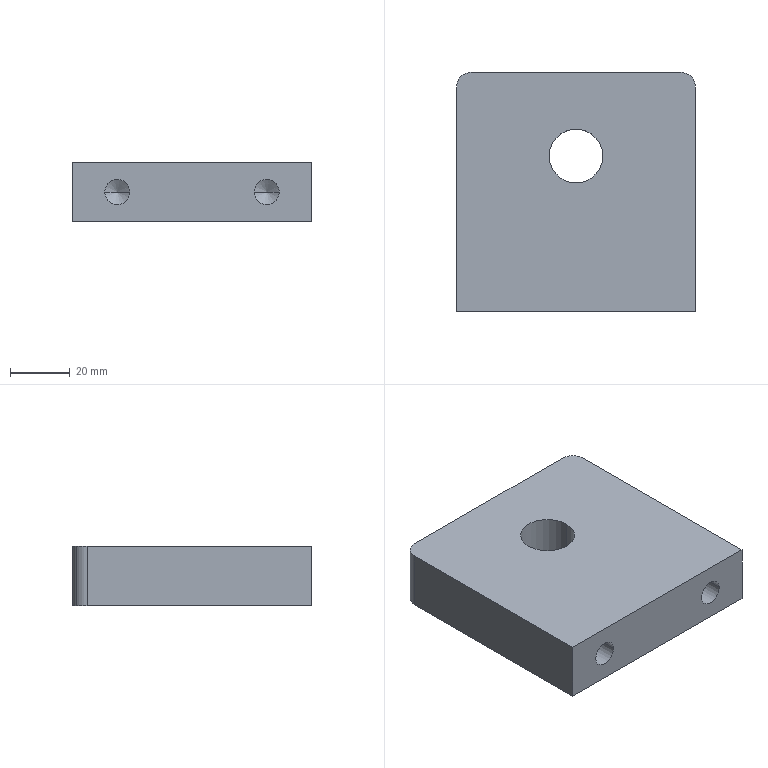Part | STEP file | DCV-000-032 | 1 solid | 20 faces | box 80 x 80 x 20 mm | volume 119595 mm3 | cylinder 10 | plane 6 | cone 4 | commonest cylinder face diameters 8.376 x4 10 x4 18 x2
STEP:
#1=CARTESIAN_POINT('',(0.,0.,0.));
#2=DIRECTION('',(0.,0.,1.));
#3=DIRECTION('',(1.,0.,0.));
#4=AXIS2_PLACEMENT_3D('',#1,#2,#3);
#5=CARTESIAN_POINT('',(40.,75.,0.));
#6=VERTEX_POINT('',#5);
#7=CARTESIAN_POINT('',(38.536,78.536,0.));
#8=VERTEX_POINT('',#7);
#9=CARTESIAN_POINT('',(35.,75.,0.));
#10=DIRECTION('',(0.,0.,1.));
#11=DIRECTION('',(0.7071,0.7071,0.));
#12=AXIS2_PLACEMENT_3D('',#9,#10,#11);
#13=CIRCLE('',#12,5.);
#14=CARTESIAN_POINT('',(35.,75.,0.));
#15=DIRECTION('',(0.,0.,1.));
#16=DIRECTION('',(0.7071,0.7071,0.));
#17=AXIS2_PLACEMENT_3D('',#14,#15,#16);
#18=CYLINDRICAL_SURFACE('',#17,5.);
#19=CARTESIAN_POINT('',(0.,0.));
#20=DIRECTION('',(1.,0.));
#21=VECTOR('',#20,1.);
#22=LINE('',#19,#21);
#23=(GEOMETRIC_REPRESENTATION_CONTEXT(2)PARAMETRIC_REPRESENTATION_CONTEXT()REPRESENTATION_CONTEXT('',''));
#24=DEFINITIONAL_REPRESENTATION('',(#22),#23);
#25=PCURVE('',#18,#24);
#26=CARTESIAN_POINT('',(0.,40.,0.));
#27=DIRECTION('',(0.,0.,1.));
#28=DIRECTION('',(1.,0.,0.));
#29=AXIS2_PLACEMENT_3D('',#26,#27,#28);
#30=PLANE('',#29);
#31=CARTESIAN_POINT('',(35.,35.));
#32=DIRECTION('',(0.7071,0.7071));
#33=AXIS2_PLACEMENT_2D('',#31,#32);
#34=CIRCLE('',#33,5.);
#35=(GEOMETRIC_REPRESENTATION_CONTEXT(2)PARAMETRIC_REPRESENTATION_CONTEXT()REPRESENTATION_CONTEXT('',''));
#36=DEFINITIONAL_REPRESENTATION('',(#34),#35);
#37=PCURVE('',#30,#36);
#38=SURFACE_CURVE('',#13,(#25,#37),.PCURVE_S1.);
#39=EDGE_CURVE('',#6,#8,#38,.T.);
#40=ORIENTED_EDGE('',*,*,#39,.T.);
#41=CARTESIAN_POINT('',(38.536,78.536,20.));
#42=VERTEX_POINT('',#41);
#43=CARTESIAN_POINT('',(38.536,78.536,0.));
#44=DIRECTION('',(0.,0.,1.));
#45=VECTOR('',#44,1.);
#46=LINE('',#43,#45);
#47=CARTESIAN_POINT('',(6.283,0.));
#48=DIRECTION('',(0.,1.));
#49=VECTOR('',#48,1.);
#50=LINE('',#47,#49);
#51=(GEOMETRIC_REPRESENTATION_CONTEXT(2)PARAMETRIC_REPRESENTATION_CONTEXT()REPRESENTATION_CONTEXT('',''));
#52=DEFINITIONAL_REPRESENTATION('',(#50),#51);
#53=PCURVE('',#18,#52);
#54=CARTESIAN_POINT('',(35.,75.,0.));
#55=DIRECTION('',(0.,0.,1.));
#56=DIRECTION('',(0.7071,0.7071,0.));
#57=AXIS2_PLACEMENT_3D('',#54,#55,#56);
#58=CYLINDRICAL_SURFACE('',#57,5.);
#59=CARTESIAN_POINT('',(0.,0.));
#60=DIRECTION('',(0.,1.));
#61=VECTOR('',#60,1.);
#62=LINE('',#59,#61);
#63=(GEOMETRIC_REPRESENTATION_CONTEXT(2)PARAMETRIC_REPRESENTATION_CONTEXT()REPRESENTATION_CONTEXT('',''));
#64=DEFINITIONAL_REPRESENTATION('',(#62),#63);
#65=PCURVE('',#58,#64);
#66=SURFACE_CURVE('',#46,(#53,#65),.PCURVE_S1.);
#67=EDGE_CURVE('',#8,#42,#66,.T.);
#68=ORIENTED_EDGE('',*,*,#67,.T.);
#69=CARTESIAN_POINT('',(40.,75.,20.));
#70=VERTEX_POINT('',#69);
#71=CARTESIAN_POINT('',(35.,75.,20.));
#72=DIRECTION('',(0.,0.,-1.));
#73=DIRECTION('',(0.7071,0.7071,0.));
#74=AXIS2_PLACEMENT_3D('',#71,#72,#73);
#75=CIRCLE('',#74,5.);
#76=CARTESIAN_POINT('',(6.283,20.));
#77=DIRECTION('',(-1.,0.));
#78=VECTOR('',#77,1.);
#79=LINE('',#76,#78);
#80=(GEOMETRIC_REPRESENTATION_CONTEXT(2)PARAMETRIC_REPRESENTATION_CONTEXT()REPRESENTATION_CONTEXT('',''));
#81=DEFINITIONAL_REPRESENTATION('',(#79),#80);
#82=PCURVE('',#18,#81);
#83=CARTESIAN_POINT('',(0.,40.,20.));
#84=DIRECTION('',(0.,0.,1.));
#85=DIRECTION('',(1.,0.,0.));
#86=AXIS2_PLACEMENT_3D('',#83,#84,#85);
#87=PLANE('',#86);
#88=CARTESIAN_POINT('',(38.536,38.536));
#89=CARTESIAN_POINT('',(44.659,32.412));
#90=CARTESIAN_POINT('',(36.294,30.17));
#91=CARTESIAN_POINT('',(27.929,27.929));
#92=CARTESIAN_POINT('',(30.17,36.294));
#93=CARTESIAN_POINT('',(32.412,44.659));
#94=CARTESIAN_POINT('',(38.536,38.536));
#95=(BOUNDED_CURVE()B_SPLINE_CURVE(2,(#88,#89,#90,#91,#92,#93,#94),.UNSPECIFIED.,.T.,.F.)B_SPLINE_CURVE_WITH_KNOTS((1,2,2,2,2,1),(-2.094,0.,2.094,4.189,6.283,8.378),.UNSPECIFIED.)CURVE()GEOMETRIC_REPRESENTATION_ITEM()RATIONAL_B_SPLINE_CURVE((1.,0.5,1.,0.5,1.,0.5,1.))REPRESENTATION_ITEM(''));
#96=(GEOMETRIC_REPRESENTATION_CONTEXT(2)PARAMETRIC_REPRESENTATION_CONTEXT()REPRESENTATION_CONTEXT('',''));
#97=DEFINITIONAL_REPRESENTATION('',(#95),#96);
#98=PCURVE('',#87,#97);
#99=SURFACE_CURVE('',#75,(#82,#98),.PCURVE_S1.);
#100=EDGE_CURVE('',#42,#70,#99,.T.);
#101=ORIENTED_EDGE('',*,*,#100,.T.);
#102=CARTESIAN_POINT('',(40.,75.,0.));
#103=DIRECTION('',(0.,0.,-1.));
#104=VECTOR('',#103,1.);
#105=LINE('',#102,#104);
#106=CARTESIAN_POINT('',(5.498,0.));
#107=DIRECTION('',(0.,-1.));
#108=VECTOR('',#107,1.);
#109=LINE('',#106,#108);
#110=(GEOMETRIC_REPRESENTATION_CONTEXT(2)PARAMETRIC_REPRESENTATION_CONTEXT()REPRESENTATION_CONTEXT('',''));
#111=DEFINITIONAL_REPRESENTATION('',(#109),#110);
#112=PCURVE('',#18,#111);
#113=CARTESIAN_POINT('',(40.,0.,0.));
#114=DIRECTION('',(1.,0.,0.));
#115=DIRECTION('',(0.,-1.,0.));
#116=AXIS2_PLACEMENT_3D('',#113,#114,#115);
#117=PLANE('',#116);
#118=CARTESIAN_POINT('',(-75.,0.));
#119=DIRECTION('',(0.,1.));
#120=VECTOR('',#119,1.);
#121=LINE('',#118,#120);
#122=(GEOMETRIC_REPRESENTATION_CONTEXT(2)PARAMETRIC_REPRESENTATION_CONTEXT()REPRESENTATION_CONTEXT('',''));
#123=DEFINITIONAL_REPRESENTATION('',(#121),#122);
#124=PCURVE('',#117,#123);
#125=SURFACE_CURVE('',#105,(#112,#124),.PCURVE_S1.);
#126=EDGE_CURVE('',#70,#6,#125,.T.);
#127=ORIENTED_EDGE('',*,*,#126,.T.);
#128=EDGE_LOOP('',(#40,#68,#101,#127));
#129=FACE_BOUND('',#128,.T.);
#130=ADVANCED_FACE('',(#129),#18,.T.);
#131=CARTESIAN_POINT('',(-35.,80.,0.));
#132=VERTEX_POINT('',#131);
#133=CARTESIAN_POINT('',(-38.536,78.536,0.));
#134=VERTEX_POINT('',#133);
#135=CARTESIAN_POINT('',(-35.,75.,0.));
#136=DIRECTION('',(0.,0.,1.));
#137=DIRECTION('',(-0.7071,0.7071,0.));
#138=AXIS2_PLACEMENT_3D('',#135,#136,#137);
#139=CIRCLE('',#138,5.);
#140=CARTESIAN_POINT('',(-35.,75.,0.));
#141=DIRECTION('',(0.,0.,1.));
#142=DIRECTION('',(-0.7071,0.7071,0.));
#143=AXIS2_PLACEMENT_3D('',#140,#141,#142);
#144=CYLINDRICAL_SURFACE('',#143,5.);
#145=CARTESIAN_POINT('',(0.,0.));
#146=DIRECTION('',(1.,0.));
#147=VECTOR('',#146,1.);
#148=LINE('',#145,#147);
#149=(GEOMETRIC_REPRESENTATION_CONTEXT(2)PARAMETRIC_REPRESENTATION_CONTEXT()REPRESENTATION_CONTEXT('',''));
#150=DEFINITIONAL_REPRESENTATION('',(#148),#149);
#151=PCURVE('',#144,#150);
#152=CARTESIAN_POINT('',(-35.,35.));
#153=DIRECTION('',(-0.7071,0.7071));
#154=AXIS2_PLACEMENT_2D('',#152,#153);
#155=CIRCLE('',#154,5.);
#156=(GEOMETRIC_REPRESENTATION_CONTEXT(2)PARAMETRIC_REPRESENTATION_CONTEXT()REPRESENTATION_CONTEXT('',''));
#157=DEFINITIONAL_REPRESENTATION('',(#155),#156);
#158=PCURVE('',#30,#157);
#159=SURFACE_CURVE('',#139,(#151,#158),.PCURVE_S1.);
#160=EDGE_CURVE('',#132,#134,#159,.T.);
#161=ORIENTED_EDGE('',*,*,#160,.T.);
#162=CARTESIAN_POINT('',(-38.536,78.536,20.));
#163=VERTEX_POINT('',#162);
#164=CARTESIAN_POINT('',(-38.536,78.536,0.));
#165=DIRECTION('',(0.,0.,1.));
#166=VECTOR('',#165,1.);
#167=LINE('',#164,#166);
#168=CARTESIAN_POINT('',(6.283,0.));
#169=DIRECTION('',(0.,1.));
#170=VECTOR('',#169,1.);
#171=LINE('',#168,#170);
#172=(GEOMETRIC_REPRESENTATION_CONTEXT(2)PARAMETRIC_REPRESENTATION_CONTEXT()REPRESENTATION_CONTEXT('',''));
#173=DEFINITIONAL_REPRESENTATION('',(#171),#172);
#174=PCURVE('',#144,#173);
#175=CARTESIAN_POINT('',(-35.,75.,0.));
#176=DIRECTION('',(0.,0.,1.));
#177=DIRECTION('',(-0.7071,0.7071,0.));
#178=AXIS2_PLACEMENT_3D('',#175,#176,#177);
#179=CYLINDRICAL_SURFACE('',#178,5.);
#180=CARTESIAN_POINT('',(0.,0.));
#181=DIRECTION('',(0.,1.));
#182=VECTOR('',#181,1.);
#183=LINE('',#180,#182);
#184=(GEOMETRIC_REPRESENTATION_CONTEXT(2)PARAMETRIC_REPRESENTATION_CONTEXT()REPRESENTATION_CONTEXT('',''));
#185=DEFINITIONAL_REPRESENTATION('',(#183),#184);
#186=PCURVE('',#179,#185);
#187=SURFACE_CURVE('',#167,(#174,#186),.PCURVE_S1.);
#188=EDGE_CURVE('',#134,#163,#187,.T.);
#189=ORIENTED_EDGE('',*,*,#188,.T.);
#190=CARTESIAN_POINT('',(-35.,80.,20.));
#191=VERTEX_POINT('',#190);
#192=CARTESIAN_POINT('',(-35.,75.,20.));
#193=DIRECTION('',(0.,0.,-1.));
#194=DIRECTION('',(-0.7071,0.7071,0.));
#195=AXIS2_PLACEMENT_3D('',#192,#193,#194);
#196=CIRCLE('',#195,5.);
#197=CARTESIAN_POINT('',(6.283,20.));
#198=DIRECTION('',(-1.,0.));
#199=VECTOR('',#198,1.);
#200=LINE('',#197,#199);
#201=(GEOMETRIC_REPRESENTATION_CONTEXT(2)PARAMETRIC_REPRESENTATION_CONTEXT()REPRESENTATION_CONTEXT('',''));
#202=DEFINITIONAL_REPRESENTATION('',(#200),#201);
#203=PCURVE('',#144,#202);
#204=CARTESIAN_POINT('',(-38.536,38.536));
#205=CARTESIAN_POINT('',(-32.412,44.659));
#206=CARTESIAN_POINT('',(-30.17,36.294));
#207=CARTESIAN_POINT('',(-27.929,27.929));
#208=CARTESIAN_POINT('',(-36.294,30.17));
#209=CARTESIAN_POINT('',(-44.659,32.412));
#210=CARTESIAN_POINT('',(-38.536,38.536));
#211=(BOUNDED_CURVE()B_SPLINE_CURVE(2,(#204,#205,#206,#207,#208,#209,#210),.UNSPECIFIED.,.T.,.F.)B_SPLINE_CURVE_WITH_KNOTS((1,2,2,2,2,1),(-2.094,0.,2.094,4.189,6.283,8.378),.UNSPECIFIED.)CURVE()GEOMETRIC_REPRESENTATION_ITEM()RATIONAL_B_SPLINE_CURVE((1.,0.5,1.,0.5,1.,0.5,1.))REPRESENTATION_ITEM(''));
#212=(GEOMETRIC_REPRESENTATION_CONTEXT(2)PARAMETRIC_REPRESENTATION_CONTEXT()REPRESENTATION_CONTEXT('',''));
#213=DEFINITIONAL_REPRESENTATION('',(#211),#212);
#214=PCURVE('',#87,#213);
#215=SURFACE_CURVE('',#196,(#203,#214),.PCURVE_S1.);
#216=EDGE_CURVE('',#163,#191,#215,.T.);
#217=ORIENTED_EDGE('',*,*,#216,.T.);
#218=CARTESIAN_POINT('',(-35.,80.,0.));
#219=DIRECTION('',(0.,0.,-1.));
#220=VECTOR('',#219,1.);
#221=LINE('',#218,#220);
#222=CARTESIAN_POINT('',(5.498,0.));
#223=DIRECTION('',(0.,-1.));
#224=VECTOR('',#223,1.);
#225=LINE('',#222,#224);
#226=(GEOMETRIC_REPRESENTATION_CONTEXT(2)PARAMETRIC_REPRESENTATION_CONTEXT()REPRESENTATION_CONTEXT('',''));
#227=DEFINITIONAL_REPRESENTATION('',(#225),#226);
#228=PCURVE('',#144,#227);
#229=CARTESIAN_POINT('',(40.,80.,0.));
#230=DIRECTION('',(0.,1.,0.));
#231=DIRECTION('',(1.,0.,0.));
#232=AXIS2_PLACEMENT_3D('',#229,#230,#231);
#233=PLANE('',#232);
#234=CARTESIAN_POINT('',(-75.,0.));
#235=DIRECTION('',(0.,1.));
#236=VECTOR('',#235,1.);
#237=LINE('',#234,#236);
#238=(GEOMETRIC_REPRESENTATION_CONTEXT(2)PARAMETRIC_REPRESENTATION_CONTEXT()REPRESENTATION_CONTEXT('',''));
#239=DEFINITIONAL_REPRESENTATION('',(#237),#238);
#240=PCURVE('',#233,#239);
#241=SURFACE_CURVE('',#221,(#228,#240),.PCURVE_S1.);
#242=EDGE_CURVE('',#191,#132,#241,.T.);
#243=ORIENTED_EDGE('',*,*,#242,.T.);
#244=EDGE_LOOP('',(#161,#189,#217,#243));
#245=FACE_BOUND('',#244,.T.);
#246=ADVANCED_FACE('',(#245),#144,.T.);
#247=CARTESIAN_POINT('',(20.812,27.3,10.));
#248=VERTEX_POINT('',#247);
#249=CARTESIAN_POINT('',(29.188,27.3,10.));
#250=VERTEX_POINT('',#249);
#251=CARTESIAN_POINT('',(25.,27.3,10.));
#252=DIRECTION('',(0.,-1.,0.));
#253=DIRECTION('',(1.,0.,0.));
#254=AXIS2_PLACEMENT_3D('',#251,#252,#253);
#255=CIRCLE('',#254,4.188);
#256=CARTESIAN_POINT('',(25.,28.558,10.));
#257=DIRECTION('',(0.,-1.,0.));
#258=DIRECTION('',(1.,0.,0.));
#259=AXIS2_PLACEMENT_3D('',#256,#257,#258);
#260=CONICAL_SURFACE('',#259,2.094,1.03);
#261=CARTESIAN_POINT('',(0.,1.258));
#262=DIRECTION('',(1.,0.));
#263=VECTOR('',#262,1.);
#264=LINE('',#261,#263);
#265=(GEOMETRIC_REPRESENTATION_CONTEXT(2)PARAMETRIC_REPRESENTATION_CONTEXT()REPRESENTATION_CONTEXT('',''));
#266=DEFINITIONAL_REPRESENTATION('',(#264),#265);
#267=PCURVE('',#260,#266);
#268=CARTESIAN_POINT('',(25.,13.65,10.));
#269=DIRECTION('',(0.,-1.,0.));
#270=DIRECTION('',(1.,0.,0.));
#271=AXIS2_PLACEMENT_3D('',#268,#269,#270);
#272=CYLINDRICAL_SURFACE('',#271,4.188);
#273=CARTESIAN_POINT('',(0.,-13.65));
#274=DIRECTION('',(1.,0.));
#275=VECTOR('',#274,1.);
#276=LINE('',#273,#275);
#277=(GEOMETRIC_REPRESENTATION_CONTEXT(2)PARAMETRIC_REPRESENTATION_CONTEXT()REPRESENTATION_CONTEXT('',''));
#278=DEFINITIONAL_REPRESENTATION('',(#276),#277);
#279=PCURVE('',#272,#278);
#280=SURFACE_CURVE('',#255,(#267,#279),.PCURVE_S1.);
#281=EDGE_CURVE('',#248,#250,#280,.T.);
#282=ORIENTED_EDGE('',*,*,#281,.F.);
#283=CARTESIAN_POINT('',(25.,29.816,10.));
#284=VERTEX_POINT('',#283);
#285=CARTESIAN_POINT('',(22.906,28.558,10.));
#286=DIRECTION('',(-0.8572,-0.515,0.));
#287=VECTOR('',#286,1.);
#288=LINE('',#285,#287);
#289=CARTESIAN_POINT('',(3.142,0.));
#290=DIRECTION('',(0.,1.));
#291=VECTOR('',#290,1.);
#292=LINE('',#289,#291);
#293=(GEOMETRIC_REPRESENTATION_CONTEXT(2)PARAMETRIC_REPRESENTATION_CONTEXT()REPRESENTATION_CONTEXT('',''));
#294=DEFINITIONAL_REPRESENTATION('',(#292),#293);
#295=PCURVE('',#260,#294);
#296=CARTESIAN_POINT('',(25.,28.558,10.));
#297=DIRECTION('',(0.,-1.,0.));
#298=DIRECTION('',(1.,0.,0.));
#299=AXIS2_PLACEMENT_3D('',#296,#297,#298);
#300=CONICAL_SURFACE('',#299,2.094,1.03);
#301=CARTESIAN_POINT('',(3.142,0.));
#302=DIRECTION('',(0.,1.));
#303=VECTOR('',#302,1.);
#304=LINE('',#301,#303);
#305=(GEOMETRIC_REPRESENTATION_CONTEXT(2)PARAMETRIC_REPRESENTATION_CONTEXT()REPRESENTATION_CONTEXT('',''));
#306=DEFINITIONAL_REPRESENTATION('',(#304),#305);
#307=PCURVE('',#300,#306);
#308=SURFACE_CURVE('',#288,(#295,#307),.PCURVE_S1.);
#309=EDGE_CURVE('',#284,#248,#308,.T.);
#310=ORIENTED_EDGE('',*,*,#309,.F.);
#311=CARTESIAN_POINT('',(27.094,28.558,10.));
#312=DIRECTION('',(0.8572,-0.515,0.));
#313=VECTOR('',#312,1.);
#314=LINE('',#311,#313);
#315=CARTESIAN_POINT('',(6.283,0.));
#316=DIRECTION('',(0.,1.));
#317=VECTOR('',#316,1.);
#318=LINE('',#315,#317);
#319=(GEOMETRIC_REPRESENTATION_CONTEXT(2)PARAMETRIC_REPRESENTATION_CONTEXT()REPRESENTATION_CONTEXT('',''));
#320=DEFINITIONAL_REPRESENTATION('',(#318),#319);
#321=PCURVE('',#260,#320);
#322=CARTESIAN_POINT('',(0.,0.));
#323=DIRECTION('',(0.,1.));
#324=VECTOR('',#323,1.);
#325=LINE('',#322,#324);
#326=(GEOMETRIC_REPRESENTATION_CONTEXT(2)PARAMETRIC_REPRESENTATION_CONTEXT()REPRESENTATION_CONTEXT('',''));
#327=DEFINITIONAL_REPRESENTATION('',(#325),#326);
#328=PCURVE('',#300,#327);
#329=SURFACE_CURVE('',#314,(#321,#328),.PCURVE_S1.);
#330=EDGE_CURVE('',#284,#250,#329,.T.);
#331=ORIENTED_EDGE('',*,*,#330,.T.);
#332=EDGE_LOOP('',(#282,#310,#331));
#333=FACE_BOUND('',#332,.F.);
#334=ADVANCED_FACE('',(#333),#260,.F.);
#335=CARTESIAN_POINT('',(29.188,0.,10.));
#336=VERTEX_POINT('',#335);
#337=CARTESIAN_POINT('',(29.188,13.65,10.));
#338=DIRECTION('',(0.,-1.,0.));
#339=VECTOR('',#338,1.);
#340=LINE('',#337,#339);
#341=CARTESIAN_POINT('',(6.283,0.));
#342=DIRECTION('',(0.,1.));
#343=VECTOR('',#342,1.);
#344=LINE('',#341,#343);
#345=(GEOMETRIC_REPRESENTATION_CONTEXT(2)PARAMETRIC_REPRESENTATION_CONTEXT()REPRESENTATION_CONTEXT('',''));
#346=DEFINITIONAL_REPRESENTATION('',(#344),#345);
#347=PCURVE('',#272,#346);
#348=CARTESIAN_POINT('',(25.,13.65,10.));
#349=DIRECTION('',(0.,-1.,0.));
#350=DIRECTION('',(1.,0.,0.));
#351=AXIS2_PLACEMENT_3D('',#348,#349,#350);
#352=CYLINDRICAL_SURFACE('',#351,4.188);
#353=CARTESIAN_POINT('',(0.,0.));
#354=DIRECTION('',(0.,1.));
#355=VECTOR('',#354,1.);
#356=LINE('',#353,#355);
#357=(GEOMETRIC_REPRESENTATION_CONTEXT(2)PARAMETRIC_REPRESENTATION_CONTEXT()REPRESENTATION_CONTEXT('',''));
#358=DEFINITIONAL_REPRESENTATION('',(#356),#357);
#359=PCURVE('',#352,#358);
#360=SURFACE_CURVE('',#340,(#347,#359),.PCURVE_S1.);
#361=EDGE_CURVE('',#250,#336,#360,.T.);
#362=ORIENTED_EDGE('',*,*,#361,.T.);
#363=CARTESIAN_POINT('',(20.812,0.,10.));
#364=VERTEX_POINT('',#363);
#365=CARTESIAN_POINT('',(25.,0.,10.));
#366=DIRECTION('',(0.,1.,0.));
#367=DIRECTION('',(1.,0.,0.));
#368=AXIS2_PLACEMENT_3D('',#365,#366,#367);
#369=CIRCLE('',#368,4.188);
#370=CARTESIAN_POINT('',(6.283,13.65));
#371=DIRECTION('',(-1.,0.));
#372=VECTOR('',#371,1.);
#373=LINE('',#370,#372);
#374=(GEOMETRIC_REPRESENTATION_CONTEXT(2)PARAMETRIC_REPRESENTATION_CONTEXT()REPRESENTATION_CONTEXT('',''));
#375=DEFINITIONAL_REPRESENTATION('',(#373),#374);
#376=PCURVE('',#272,#375);
#377=CARTESIAN_POINT('',(-40.,0.,0.));
#378=DIRECTION('',(0.,-1.,0.));
#379=DIRECTION('',(0.,0.,-1.));
#380=AXIS2_PLACEMENT_3D('',#377,#378,#379);
#381=PLANE('',#380);
#382=CARTESIAN_POINT('',(-10.,69.188));
#383=CARTESIAN_POINT('',(-2.746,69.188));
#384=CARTESIAN_POINT('',(-6.373,62.906));
#385=CARTESIAN_POINT('',(-10.,56.624));
#386=CARTESIAN_POINT('',(-13.627,62.906));
#387=CARTESIAN_POINT('',(-17.254,69.188));
#388=CARTESIAN_POINT('',(-10.,69.188));
#389=(BOUNDED_CURVE()B_SPLINE_CURVE(2,(#382,#383,#384,#385,#386,#387,#388),.UNSPECIFIED.,.T.,.F.)B_SPLINE_CURVE_WITH_KNOTS((1,2,2,2,2,1),(-2.094,0.,2.094,4.189,6.283,8.378),.UNSPECIFIED.)CURVE()GEOMETRIC_REPRESENTATION_ITEM()RATIONAL_B_SPLINE_CURVE((1.,0.5,1.,0.5,1.,0.5,1.))REPRESENTATION_ITEM(''));
#390=(GEOMETRIC_REPRESENTATION_CONTEXT(2)PARAMETRIC_REPRESENTATION_CONTEXT()REPRESENTATION_CONTEXT('',''));
#391=DEFINITIONAL_REPRESENTATION('',(#389),#390);
#392=PCURVE('',#381,#391);
#393=SURFACE_CURVE('',#369,(#376,#392),.PCURVE_S1.);
#394=EDGE_CURVE('',#336,#364,#393,.T.);
#395=ORIENTED_EDGE('',*,*,#394,.T.);
#396=CARTESIAN_POINT('',(20.812,13.65,10.));
#397=DIRECTION('',(0.,-1.,0.));
#398=VECTOR('',#397,1.);
#399=LINE('',#396,#398);
#400=CARTESIAN_POINT('',(3.142,0.));
#401=DIRECTION('',(0.,1.));
#402=VECTOR('',#401,1.);
#403=LINE('',#400,#402);
#404=(GEOMETRIC_REPRESENTATION_CONTEXT(2)PARAMETRIC_REPRESENTATION_CONTEXT()REPRESENTATION_CONTEXT('',''));
#405=DEFINITIONAL_REPRESENTATION('',(#403),#404);
#406=PCURVE('',#272,#405);
#407=CARTESIAN_POINT('',(3.142,0.));
#408=DIRECTION('',(0.,1.));
#409=VECTOR('',#408,1.);
#410=LINE('',#407,#409);
#411=(GEOMETRIC_REPRESENTATION_CONTEXT(2)PARAMETRIC_REPRESENTATION_CONTEXT()REPRESENTATION_CONTEXT('',''));
#412=DEFINITIONAL_REPRESENTATION('',(#410),#411);
#413=PCURVE('',#352,#412);
#414=SURFACE_CURVE('',#399,(#406,#413),.PCURVE_S1.);
#415=EDGE_CURVE('',#248,#364,#414,.T.);
#416=ORIENTED_EDGE('',*,*,#415,.F.);
#417=ORIENTED_EDGE('',*,*,#281,.T.);
#418=EDGE_LOOP('',(#362,#395,#416,#417));
#419=FACE_BOUND('',#418,.F.);
#420=ADVANCED_FACE('',(#419),#272,.F.);
#421=CARTESIAN_POINT('',(-29.188,27.3,10.));
#422=VERTEX_POINT('',#421);
#423=CARTESIAN_POINT('',(-20.812,27.3,10.));
#424=VERTEX_POINT('',#423);
#425=CARTESIAN_POINT('',(-25.,27.3,10.));
#426=DIRECTION('',(0.,-1.,0.));
#427=DIRECTION('',(1.,0.,0.));
#428=AXIS2_PLACEMENT_3D('',#425,#426,#427);
#429=CIRCLE('',#428,4.188);
#430=CARTESIAN_POINT('',(-25.,28.558,10.));
#431=DIRECTION('',(0.,-1.,0.));
#432=DIRECTION('',(1.,0.,0.));
#433=AXIS2_PLACEMENT_3D('',#430,#431,#432);
#434=CONICAL_SURFACE('',#433,2.094,1.03);
#435=CARTESIAN_POINT('',(0.,1.258));
#436=DIRECTION('',(1.,0.));
#437=VECTOR('',#436,1.);
#438=LINE('',#435,#437);
#439=(GEOMETRIC_REPRESENTATION_CONTEXT(2)PARAMETRIC_REPRESENTATION_CONTEXT()REPRESENTATION_CONTEXT('',''));
#440=DEFINITIONAL_REPRESENTATION('',(#438),#439);
#441=PCURVE('',#434,#440);
#442=CARTESIAN_POINT('',(-25.,13.65,10.));
#443=DIRECTION('',(0.,-1.,0.));
#444=DIRECTION('',(1.,0.,0.));
#445=AXIS2_PLACEMENT_3D('',#442,#443,#444);
#446=CYLINDRICAL_SURFACE('',#445,4.188);
#447=CARTESIAN_POINT('',(0.,-13.65));
#448=DIRECTION('',(1.,0.));
#449=VECTOR('',#448,1.);
#450=LINE('',#447,#449);
#451=(GEOMETRIC_REPRESENTATION_CONTEXT(2)PARAMETRIC_REPRESENTATION_CONTEXT()REPRESENTATION_CONTEXT('',''));
#452=DEFINITIONAL_REPRESENTATION('',(#450),#451);
#453=PCURVE('',#446,#452);
#454=SURFACE_CURVE('',#429,(#441,#453),.PCURVE_S1.);
#455=EDGE_CURVE('',#422,#424,#454,.T.);
#456=ORIENTED_EDGE('',*,*,#455,.F.);
#457=CARTESIAN_POINT('',(-25.,29.816,10.));
#458=VERTEX_POINT('',#457);
#459=CARTESIAN_POINT('',(-27.094,28.558,10.));
#460=DIRECTION('',(-0.8572,-0.515,0.));
#461=VECTOR('',#460,1.);
#462=LINE('',#459,#461);
#463=CARTESIAN_POINT('',(3.142,0.));
#464=DIRECTION('',(0.,1.));
#465=VECTOR('',#464,1.);
#466=LINE('',#463,#465);
#467=(GEOMETRIC_REPRESENTATION_CONTEXT(2)PARAMETRIC_REPRESENTATION_CONTEXT()REPRESENTATION_CONTEXT('',''));
#468=DEFINITIONAL_REPRESENTATION('',(#466),#467);
#469=PCURVE('',#434,#468);
#470=CARTESIAN_POINT('',(-25.,28.558,10.));
#471=DIRECTION('',(0.,-1.,0.));
#472=DIRECTION('',(1.,0.,0.));
#473=AXIS2_PLACEMENT_3D('',#470,#471,#472);
#474=CONICAL_SURFACE('',#473,2.094,1.03);
#475=CARTESIAN_POINT('',(3.142,0.));
#476=DIRECTION('',(0.,1.));
#477=VECTOR('',#476,1.);
#478=LINE('',#475,#477);
#479=(GEOMETRIC_REPRESENTATION_CONTEXT(2)PARAMETRIC_REPRESENTATION_CONTEXT()REPRESENTATION_CONTEXT('',''));
#480=DEFINITIONAL_REPRESENTATION('',(#478),#479);
#481=PCURVE('',#474,#480);
#482=SURFACE_CURVE('',#462,(#469,#481),.PCURVE_S1.);
#483=EDGE_CURVE('',#458,#422,#482,.T.);
#484=ORIENTED_EDGE('',*,*,#483,.F.);
#485=CARTESIAN_POINT('',(-22.906,28.558,10.));
#486=DIRECTION('',(0.8572,-0.515,0.));
#487=VECTOR('',#486,1.);
#488=LINE('',#485,#487);
#489=CARTESIAN_POINT('',(6.283,0.));
#490=DIRECTION('',(0.,1.));
#491=VECTOR('',#490,1.);
#492=LINE('',#489,#491);
#493=(GEOMETRIC_REPRESENTATION_CONTEXT(2)PARAMETRIC_REPRESENTATION_CONTEXT()REPRESENTATION_CONTEXT('',''));
#494=DEFINITIONAL_REPRESENTATION('',(#492),#493);
#495=PCURVE('',#434,#494);
#496=CARTESIAN_POINT('',(0.,0.));
#497=DIRECTION('',(0.,1.));
#498=VECTOR('',#497,1.);
#499=LINE('',#496,#498);
#500=(GEOMETRIC_REPRESENTATION_CONTEXT(2)PARAMETRIC_REPRESENTATION_CONTEXT()REPRESENTATION_CONTEXT('',''));
#501=DEFINITIONAL_REPRESENTATION('',(#499),#500);
#502=PCURVE('',#474,#501);
#503=SURFACE_CURVE('',#488,(#495,#502),.PCURVE_S1.);
#504=EDGE_CURVE('',#458,#424,#503,.T.);
#505=ORIENTED_EDGE('',*,*,#504,.T.);
#506=EDGE_LOOP('',(#456,#484,#505));
#507=FACE_BOUND('',#506,.F.);
#508=ADVANCED_FACE('',(#507),#434,.F.);
#509=CARTESIAN_POINT('',(-20.812,0.,10.));
#510=VERTEX_POINT('',#509);
#511=CARTESIAN_POINT('',(-20.812,13.65,10.));
#512=DIRECTION('',(0.,-1.,0.));
#513=VECTOR('',#512,1.);
#514=LINE('',#511,#513);
#515=CARTESIAN_POINT('',(6.283,0.));
#516=DIRECTION('',(0.,1.));
#517=VECTOR('',#516,1.);
#518=LINE('',#515,#517);
#519=(GEOMETRIC_REPRESENTATION_CONTEXT(2)PARAMETRIC_REPRESENTATION_CONTEXT()REPRESENTATION_CONTEXT('',''));
#520=DEFINITIONAL_REPRESENTATION('',(#518),#519);
#521=PCURVE('',#446,#520);
#522=CARTESIAN_POINT('',(-25.,13.65,10.));
#523=DIRECTION('',(0.,-1.,0.));
#524=DIRECTION('',(1.,0.,0.));
#525=AXIS2_PLACEMENT_3D('',#522,#523,#524);
#526=CYLINDRICAL_SURFACE('',#525,4.188);
#527=CARTESIAN_POINT('',(0.,0.));
#528=DIRECTION('',(0.,1.));
#529=VECTOR('',#528,1.);
#530=LINE('',#527,#529);
#531=(GEOMETRIC_REPRESENTATION_CONTEXT(2)PARAMETRIC_REPRESENTATION_CONTEXT()REPRESENTATION_CONTEXT('',''));
#532=DEFINITIONAL_REPRESENTATION('',(#530),#531);
#533=PCURVE('',#526,#532);
#534=SURFACE_CURVE('',#514,(#521,#533),.PCURVE_S1.);
#535=EDGE_CURVE('',#424,#510,#534,.T.);
#536=ORIENTED_EDGE('',*,*,#535,.T.);
#537=CARTESIAN_POINT('',(-29.188,0.,10.));
#538=VERTEX_POINT('',#537);
#539=CARTESIAN_POINT('',(-25.,0.,10.));
#540=DIRECTION('',(0.,1.,0.));
#541=DIRECTION('',(1.,0.,0.));
#542=AXIS2_PLACEMENT_3D('',#539,#540,#541);
#543=CIRCLE('',#542,4.188);
#544=CARTESIAN_POINT('',(6.283,13.65));
#545=DIRECTION('',(-1.,0.));
#546=VECTOR('',#545,1.);
#547=LINE('',#544,#546);
#548=(GEOMETRIC_REPRESENTATION_CONTEXT(2)PARAMETRIC_REPRESENTATION_CONTEXT()REPRESENTATION_CONTEXT('',''));
#549=DEFINITIONAL_REPRESENTATION('',(#547),#548);
#550=PCURVE('',#446,#549);
#551=CARTESIAN_POINT('',(-10.,19.188));
#552=CARTESIAN_POINT('',(-2.746,19.188));
#553=CARTESIAN_POINT('',(-6.373,12.906));
#554=CARTESIAN_POINT('',(-10.,6.624));
#555=CARTESIAN_POINT('',(-13.627,12.906));
#556=CARTESIAN_POINT('',(-17.254,19.188));
#557=CARTESIAN_POINT('',(-10.,19.188));
#558=(BOUNDED_CURVE()B_SPLINE_CURVE(2,(#551,#552,#553,#554,#555,#556,#557),.UNSPECIFIED.,.T.,.F.)B_SPLINE_CURVE_WITH_KNOTS((1,2,2,2,2,1),(-2.094,0.,2.094,4.189,6.283,8.378),.UNSPECIFIED.)CURVE()GEOMETRIC_REPRESENTATION_ITEM()RATIONAL_B_SPLINE_CURVE((1.,0.5,1.,0.5,1.,0.5,1.))REPRESENTATION_ITEM(''));
#559=(GEOMETRIC_REPRESENTATION_CONTEXT(2)PARAMETRIC_REPRESENTATION_CONTEXT()REPRESENTATION_CONTEXT('',''));
#560=DEFINITIONAL_REPRESENTATION('',(#558),#559);
#561=PCURVE('',#381,#560);
#562=SURFACE_CURVE('',#543,(#550,#561),.PCURVE_S1.);
#563=EDGE_CURVE('',#510,#538,#562,.T.);
#564=ORIENTED_EDGE('',*,*,#563,.T.);
#565=CARTESIAN_POINT('',(-29.188,13.65,10.));
#566=DIRECTION('',(0.,-1.,0.));
#567=VECTOR('',#566,1.);
#568=LINE('',#565,#567);
#569=CARTESIAN_POINT('',(3.142,0.));
#570=DIRECTION('',(0.,1.));
#571=VECTOR('',#570,1.);
#572=LINE('',#569,#571);
#573=(GEOMETRIC_REPRESENTATION_CONTEXT(2)PARAMETRIC_REPRESENTATION_CONTEXT()REPRESENTATION_CONTEXT('',''));
#574=DEFINITIONAL_REPRESENTATION('',(#572),#573);
#575=PCURVE('',#446,#574);
#576=CARTESIAN_POINT('',(3.142,0.));
#577=DIRECTION('',(0.,1.));
#578=VECTOR('',#577,1.);
#579=LINE('',#576,#578);
#580=(GEOMETRIC_REPRESENTATION_CONTEXT(2)PARAMETRIC_REPRESENTATION_CONTEXT()REPRESENTATION_CONTEXT('',''));
#581=DEFINITIONAL_REPRESENTATION('',(#579),#580);
#582=PCURVE('',#526,#581);
#583=SURFACE_CURVE('',#568,(#575,#582),.PCURVE_S1.);
#584=EDGE_CURVE('',#422,#538,#583,.T.);
#585=ORIENTED_EDGE('',*,*,#584,.F.);
#586=ORIENTED_EDGE('',*,*,#455,.T.);
#587=EDGE_LOOP('',(#536,#564,#585,#586));
#588=FACE_BOUND('',#587,.F.);
#589=ADVANCED_FACE('',(#588),#446,.F.);
#590=CARTESIAN_POINT('',(9.,52.,0.));
#591=VERTEX_POINT('',#590);
#592=CARTESIAN_POINT('',(9.,52.,20.));
#593=VERTEX_POINT('',#592);
#594=CARTESIAN_POINT('',(9.,52.,-94.891));
#595=DIRECTION('',(0.,0.,1.));
#596=VECTOR('',#595,1.);
#597=LINE('',#594,#596);
#598=CARTESIAN_POINT('',(0.,52.,-94.891));
#599=DIRECTION('',(0.,0.,1.));
#600=DIRECTION('',(1.,0.,0.));
#601=AXIS2_PLACEMENT_3D('',#598,#599,#600);
#602=CYLINDRICAL_SURFACE('',#601,9.);
#603=CARTESIAN_POINT('',(6.283,0.));
#604=DIRECTION('',(0.,1.));
#605=VECTOR('',#604,1.);
#606=LINE('',#603,#605);
#607=(GEOMETRIC_REPRESENTATION_CONTEXT(2)PARAMETRIC_REPRESENTATION_CONTEXT()REPRESENTATION_CONTEXT('',''));
#608=DEFINITIONAL_REPRESENTATION('',(#606),#607);
#609=PCURVE('',#602,#608);
#610=CARTESIAN_POINT('',(0.,52.,-94.891));
#611=DIRECTION('',(0.,0.,1.));
#612=DIRECTION('',(1.,0.,0.));
#613=AXIS2_PLACEMENT_3D('',#610,#611,#612);
#614=CYLINDRICAL_SURFACE('',#613,9.);
#615=CARTESIAN_POINT('',(0.,0.));
#616=DIRECTION('',(0.,1.));
#617=VECTOR('',#616,1.);
#618=LINE('',#615,#617);
#619=(GEOMETRIC_REPRESENTATION_CONTEXT(2)PARAMETRIC_REPRESENTATION_CONTEXT()REPRESENTATION_CONTEXT('',''));
#620=DEFINITIONAL_REPRESENTATION('',(#618),#619);
#621=PCURVE('',#614,#620);
#622=SURFACE_CURVE('',#597,(#609,#621),.PCURVE_S1.);
#623=EDGE_CURVE('',#591,#593,#622,.T.);
#624=ORIENTED_EDGE('',*,*,#623,.T.);
#625=CARTESIAN_POINT('',(-9.,52.,20.));
#626=VERTEX_POINT('',#625);
#627=CARTESIAN_POINT('',(0.,52.,20.));
#628=DIRECTION('',(0.,0.,-1.));
#629=DIRECTION('',(1.,0.,0.));
#630=AXIS2_PLACEMENT_3D('',#627,#628,#629);
#631=CIRCLE('',#630,9.);
#632=CARTESIAN_POINT('',(6.283,114.891));
#633=DIRECTION('',(-1.,0.));
#634=VECTOR('',#633,1.);
#635=LINE('',#632,#634);
#636=(GEOMETRIC_REPRESENTATION_CONTEXT(2)PARAMETRIC_REPRESENTATION_CONTEXT()REPRESENTATION_CONTEXT('',''));
#637=DEFINITIONAL_REPRESENTATION('',(#635),#636);
#638=PCURVE('',#602,#637);
#639=CARTESIAN_POINT('',(9.,12.));
#640=CARTESIAN_POINT('',(9.,-3.588));
#641=CARTESIAN_POINT('',(-4.5,4.206));
#642=CARTESIAN_POINT('',(-18.,12.));
#643=CARTESIAN_POINT('',(-4.5,19.794));
#644=CARTESIAN_POINT('',(9.,27.588));
#645=CARTESIAN_POINT('',(9.,12.));
#646=(BOUNDED_CURVE()B_SPLINE_CURVE(2,(#639,#640,#641,#642,#643,#644,#645),.UNSPECIFIED.,.T.,.F.)B_SPLINE_CURVE_WITH_KNOTS((1,2,2,2,2,1),(-2.094,0.,2.094,4.189,6.283,8.378),.UNSPECIFIED.)CURVE()GEOMETRIC_REPRESENTATION_ITEM()RATIONAL_B_SPLINE_CURVE((1.,0.5,1.,0.5,1.,0.5,1.))REPRESENTATION_ITEM(''));
#647=(GEOMETRIC_REPRESENTATION_CONTEXT(2)PARAMETRIC_REPRESENTATION_CONTEXT()REPRESENTATION_CONTEXT('',''));
#648=DEFINITIONAL_REPRESENTATION('',(#646),#647);
#649=PCURVE('',#87,#648);
#650=SURFACE_CURVE('',#631,(#638,#649),.PCURVE_S1.);
#651=EDGE_CURVE('',#593,#626,#650,.T.);
#652=ORIENTED_EDGE('',*,*,#651,.T.);
#653=CARTESIAN_POINT('',(-9.,52.,0.));
#654=VERTEX_POINT('',#653);
#655=CARTESIAN_POINT('',(-9.,52.,-94.891));
#656=DIRECTION('',(0.,0.,1.));
#657=VECTOR('',#656,1.);
#658=LINE('',#655,#657);
#659=CARTESIAN_POINT('',(3.142,0.));
#660=DIRECTION('',(0.,1.));
#661=VECTOR('',#660,1.);
#662=LINE('',#659,#661);
#663=(GEOMETRIC_REPRESENTATION_CONTEXT(2)PARAMETRIC_REPRESENTATION_CONTEXT()REPRESENTATION_CONTEXT('',''));
#664=DEFINITIONAL_REPRESENTATION('',(#662),#663);
#665=PCURVE('',#602,#664);
#666=CARTESIAN_POINT('',(3.142,0.));
#667=DIRECTION('',(0.,1.));
#668=VECTOR('',#667,1.);
#669=LINE('',#666,#668);
#670=(GEOMETRIC_REPRESENTATION_CONTEXT(2)PARAMETRIC_REPRESENTATION_CONTEXT()REPRESENTATION_CONTEXT('',''));
#671=DEFINITIONAL_REPRESENTATION('',(#669),#670);
#672=PCURVE('',#614,#671);
#673=SURFACE_CURVE('',#658,(#665,#672),.PCURVE_S1.);
#674=EDGE_CURVE('',#654,#626,#673,.T.);
#675=ORIENTED_EDGE('',*,*,#674,.F.);
#676=CARTESIAN_POINT('',(0.,52.,0.));
#677=DIRECTION('',(0.,0.,1.));
#678=DIRECTION('',(1.,0.,0.));
#679=AXIS2_PLACEMENT_3D('',#676,#677,#678);
#680=CIRCLE('',#679,9.);
#681=CARTESIAN_POINT('',(0.,94.891));
#682=DIRECTION('',(1.,0.));
#683=VECTOR('',#682,1.);
#684=LINE('',#681,#683);
#685=(GEOMETRIC_REPRESENTATION_CONTEXT(2)PARAMETRIC_REPRESENTATION_CONTEXT()REPRESENTATION_CONTEXT('',''));
#686=DEFINITIONAL_REPRESENTATION('',(#684),#685);
#687=PCURVE('',#602,#686);
#688=CARTESIAN_POINT('',(0.,12.));
#689=DIRECTION('',(1.,0.));
#690=AXIS2_PLACEMENT_2D('',#688,#689);
#691=CIRCLE('',#690,9.);
#692=(GEOMETRIC_REPRESENTATION_CONTEXT(2)PARAMETRIC_REPRESENTATION_CONTEXT()REPRESENTATION_CONTEXT('',''));
#693=DEFINITIONAL_REPRESENTATION('',(#691),#692);
#694=PCURVE('',#30,#693);
#695=SURFACE_CURVE('',#680,(#687,#694),.PCURVE_S1.);
#696=EDGE_CURVE('',#654,#591,#695,.T.);
#697=ORIENTED_EDGE('',*,*,#696,.T.);
#698=EDGE_LOOP('',(#624,#652,#675,#697));
#699=FACE_BOUND('',#698,.F.);
#700=ADVANCED_FACE('',(#699),#602,.F.);
#701=ORIENTED_EDGE('',*,*,#651,.T.);
#702=CARTESIAN_POINT('',(0.,52.,20.));
#703=DIRECTION('',(0.,0.,-1.));
#704=DIRECTION('',(1.,0.,0.));
#705=AXIS2_PLACEMENT_3D('',#702,#703,#704);
#706=CIRCLE('',#705,9.);
#707=CARTESIAN_POINT('',(9.,12.));
#708=CARTESIAN_POINT('',(9.,-3.588));
#709=CARTESIAN_POINT('',(-4.5,4.206));
#710=CARTESIAN_POINT('',(-18.,12.));
#711=CARTESIAN_POINT('',(-4.5,19.794));
#712=CARTESIAN_POINT('',(9.,27.588));
#713=CARTESIAN_POINT('',(9.,12.));
#714=(BOUNDED_CURVE()B_SPLINE_CURVE(2,(#707,#708,#709,#710,#711,#712,#713),.UNSPECIFIED.,.T.,.F.)B_SPLINE_CURVE_WITH_KNOTS((1,2,2,2,2,1),(-2.094,0.,2.094,4.189,6.283,8.378),.UNSPECIFIED.)CURVE()GEOMETRIC_REPRESENTATION_ITEM()RATIONAL_B_SPLINE_CURVE((1.,0.5,1.,0.5,1.,0.5,1.))REPRESENTATION_ITEM(''));
#715=(GEOMETRIC_REPRESENTATION_CONTEXT(2)PARAMETRIC_REPRESENTATION_CONTEXT()REPRESENTATION_CONTEXT('',''));
#716=DEFINITIONAL_REPRESENTATION('',(#714),#715);
#717=PCURVE('',#87,#716);
#718=CARTESIAN_POINT('',(6.283,114.891));
#719=DIRECTION('',(-1.,0.));
#720=VECTOR('',#719,1.);
#721=LINE('',#718,#720);
#722=(GEOMETRIC_REPRESENTATION_CONTEXT(2)PARAMETRIC_REPRESENTATION_CONTEXT()REPRESENTATION_CONTEXT('',''));
#723=DEFINITIONAL_REPRESENTATION('',(#721),#722);
#724=PCURVE('',#614,#723);
#725=SURFACE_CURVE('',#706,(#717,#724),.PCURVE_S1.);
#726=EDGE_CURVE('',#626,#593,#725,.T.);
#727=ORIENTED_EDGE('',*,*,#726,.T.);
#728=EDGE_LOOP('',(#701,#727));
#729=FACE_BOUND('',#728,.T.);
#730=CARTESIAN_POINT('',(35.,80.,20.));
#731=VERTEX_POINT('',#730);
#732=CARTESIAN_POINT('',(35.,75.,20.));
#733=DIRECTION('',(0.,0.,-1.));
#734=DIRECTION('',(0.7071,0.7071,0.));
#735=AXIS2_PLACEMENT_3D('',#732,#733,#734);
#736=CIRCLE('',#735,5.);
#737=CARTESIAN_POINT('',(38.536,38.536));
#738=CARTESIAN_POINT('',(44.659,32.412));
#739=CARTESIAN_POINT('',(36.294,30.17));
#740=CARTESIAN_POINT('',(27.929,27.929));
#741=CARTESIAN_POINT('',(30.17,36.294));
#742=CARTESIAN_POINT('',(32.412,44.659));
#743=CARTESIAN_POINT('',(38.536,38.536));
#744=(BOUNDED_CURVE()B_SPLINE_CURVE(2,(#737,#738,#739,#740,#741,#742,#743),.UNSPECIFIED.,.T.,.F.)B_SPLINE_CURVE_WITH_KNOTS((1,2,2,2,2,1),(-2.094,0.,2.094,4.189,6.283,8.378),.UNSPECIFIED.)CURVE()GEOMETRIC_REPRESENTATION_ITEM()RATIONAL_B_SPLINE_CURVE((1.,0.5,1.,0.5,1.,0.5,1.))REPRESENTATION_ITEM(''));
#745=(GEOMETRIC_REPRESENTATION_CONTEXT(2)PARAMETRIC_REPRESENTATION_CONTEXT()REPRESENTATION_CONTEXT('',''));
#746=DEFINITIONAL_REPRESENTATION('',(#744),#745);
#747=PCURVE('',#87,#746);
#748=CARTESIAN_POINT('',(6.283,20.));
#749=DIRECTION('',(-1.,0.));
#750=VECTOR('',#749,1.);
#751=LINE('',#748,#750);
#752=(GEOMETRIC_REPRESENTATION_CONTEXT(2)PARAMETRIC_REPRESENTATION_CONTEXT()REPRESENTATION_CONTEXT('',''));
#753=DEFINITIONAL_REPRESENTATION('',(#751),#752);
#754=PCURVE('',#58,#753);
#755=SURFACE_CURVE('',#736,(#747,#754),.PCURVE_S1.);
#756=EDGE_CURVE('',#731,#42,#755,.T.);
#757=ORIENTED_EDGE('',*,*,#756,.F.);
#758=CARTESIAN_POINT('',(40.,80.,20.));
#759=DIRECTION('',(-1.,0.,0.));
#760=VECTOR('',#759,1.);
#761=LINE('',#758,#760);
#762=CARTESIAN_POINT('',(40.,40.));
#763=DIRECTION('',(-1.,0.));
#764=VECTOR('',#763,1.);
#765=LINE('',#762,#764);
#766=(GEOMETRIC_REPRESENTATION_CONTEXT(2)PARAMETRIC_REPRESENTATION_CONTEXT()REPRESENTATION_CONTEXT('',''));
#767=DEFINITIONAL_REPRESENTATION('',(#765),#766);
#768=PCURVE('',#87,#767);
#769=CARTESIAN_POINT('',(0.,-20.));
#770=DIRECTION('',(-1.,0.));
#771=VECTOR('',#770,1.);
#772=LINE('',#769,#771);
#773=(GEOMETRIC_REPRESENTATION_CONTEXT(2)PARAMETRIC_REPRESENTATION_CONTEXT()REPRESENTATION_CONTEXT('',''));
#774=DEFINITIONAL_REPRESENTATION('',(#772),#773);
#775=PCURVE('',#233,#774);
#776=SURFACE_CURVE('',#761,(#768,#775),.PCURVE_S1.);
#777=EDGE_CURVE('',#731,#191,#776,.T.);
#778=ORIENTED_EDGE('',*,*,#777,.T.);
#779=ORIENTED_EDGE('',*,*,#216,.F.);
#780=CARTESIAN_POINT('',(-40.,75.,20.));
#781=VERTEX_POINT('',#780);
#782=CARTESIAN_POINT('',(-35.,75.,20.));
#783=DIRECTION('',(0.,0.,-1.));
#784=DIRECTION('',(-0.7071,0.7071,0.));
#785=AXIS2_PLACEMENT_3D('',#782,#783,#784);
#786=CIRCLE('',#785,5.);
#787=CARTESIAN_POINT('',(-38.536,38.536));
#788=CARTESIAN_POINT('',(-32.412,44.659));
#789=CARTESIAN_POINT('',(-30.17,36.294));
#790=CARTESIAN_POINT('',(-27.929,27.929));
#791=CARTESIAN_POINT('',(-36.294,30.17));
#792=CARTESIAN_POINT('',(-44.659,32.412));
#793=CARTESIAN_POINT('',(-38.536,38.536));
#794=(BOUNDED_CURVE()B_SPLINE_CURVE(2,(#787,#788,#789,#790,#791,#792,#793),.UNSPECIFIED.,.T.,.F.)B_SPLINE_CURVE_WITH_KNOTS((1,2,2,2,2,1),(-2.094,0.,2.094,4.189,6.283,8.378),.UNSPECIFIED.)CURVE()GEOMETRIC_REPRESENTATION_ITEM()RATIONAL_B_SPLINE_CURVE((1.,0.5,1.,0.5,1.,0.5,1.))REPRESENTATION_ITEM(''));
#795=(GEOMETRIC_REPRESENTATION_CONTEXT(2)PARAMETRIC_REPRESENTATION_CONTEXT()REPRESENTATION_CONTEXT('',''));
#796=DEFINITIONAL_REPRESENTATION('',(#794),#795);
#797=PCURVE('',#87,#796);
#798=CARTESIAN_POINT('',(6.283,20.));
#799=DIRECTION('',(-1.,0.));
#800=VECTOR('',#799,1.);
#801=LINE('',#798,#800);
#802=(GEOMETRIC_REPRESENTATION_CONTEXT(2)PARAMETRIC_REPRESENTATION_CONTEXT()REPRESENTATION_CONTEXT('',''));
#803=DEFINITIONAL_REPRESENTATION('',(#801),#802);
#804=PCURVE('',#179,#803);
#805=SURFACE_CURVE('',#786,(#797,#804),.PCURVE_S1.);
#806=EDGE_CURVE('',#781,#163,#805,.T.);
#807=ORIENTED_EDGE('',*,*,#806,.F.);
#808=CARTESIAN_POINT('',(-40.,0.,20.));
#809=VERTEX_POINT('',#808);
#810=CARTESIAN_POINT('',(-40.,80.,20.));
#811=DIRECTION('',(0.,-1.,0.));
#812=VECTOR('',#811,1.);
#813=LINE('',#810,#812);
#814=CARTESIAN_POINT('',(-40.,40.));
#815=DIRECTION('',(0.,-1.));
#816=VECTOR('',#815,1.);
#817=LINE('',#814,#816);
#818=(GEOMETRIC_REPRESENTATION_CONTEXT(2)PARAMETRIC_REPRESENTATION_CONTEXT()REPRESENTATION_CONTEXT('',''));
#819=DEFINITIONAL_REPRESENTATION('',(#817),#818);
#820=PCURVE('',#87,#819);
#821=CARTESIAN_POINT('',(-40.,80.,0.));
#822=DIRECTION('',(-1.,0.,0.));
#823=DIRECTION('',(0.,1.,0.));
#824=AXIS2_PLACEMENT_3D('',#821,#822,#823);
#825=PLANE('',#824);
#826=CARTESIAN_POINT('',(0.,-20.));
#827=DIRECTION('',(-1.,0.));
#828=VECTOR('',#827,1.);
#829=LINE('',#826,#828);
#830=(GEOMETRIC_REPRESENTATION_CONTEXT(2)PARAMETRIC_REPRESENTATION_CONTEXT()REPRESENTATION_CONTEXT('',''));
#831=DEFINITIONAL_REPRESENTATION('',(#829),#830);
#832=PCURVE('',#825,#831);
#833=SURFACE_CURVE('',#813,(#820,#832),.PCURVE_S1.);
#834=EDGE_CURVE('',#781,#809,#833,.T.);
#835=ORIENTED_EDGE('',*,*,#834,.T.);
#836=CARTESIAN_POINT('',(40.,0.,20.));
#837=VERTEX_POINT('',#836);
#838=CARTESIAN_POINT('',(-40.,0.,20.));
#839=DIRECTION('',(1.,0.,0.));
#840=VECTOR('',#839,1.);
#841=LINE('',#838,#840);
#842=CARTESIAN_POINT('',(-40.,-40.));
#843=DIRECTION('',(1.,0.));
#844=VECTOR('',#843,1.);
#845=LINE('',#842,#844);
#846=(GEOMETRIC_REPRESENTATION_CONTEXT(2)PARAMETRIC_REPRESENTATION_CONTEXT()REPRESENTATION_CONTEXT('',''));
#847=DEFINITIONAL_REPRESENTATION('',(#845),#846);
#848=PCURVE('',#87,#847);
#849=CARTESIAN_POINT('',(-20.,0.));
#850=DIRECTION('',(0.,1.));
#851=VECTOR('',#850,1.);
#852=LINE('',#849,#851);
#853=(GEOMETRIC_REPRESENTATION_CONTEXT(2)PARAMETRIC_REPRESENTATION_CONTEXT()REPRESENTATION_CONTEXT('',''));
#854=DEFINITIONAL_REPRESENTATION('',(#852),#853);
#855=PCURVE('',#381,#854);
#856=SURFACE_CURVE('',#841,(#848,#855),.PCURVE_S1.);
#857=EDGE_CURVE('',#809,#837,#856,.T.);
#858=ORIENTED_EDGE('',*,*,#857,.T.);
#859=CARTESIAN_POINT('',(40.,0.,20.));
#860=DIRECTION('',(0.,1.,0.));
#861=VECTOR('',#860,1.);
#862=LINE('',#859,#861);
#863=CARTESIAN_POINT('',(40.,-40.));
#864=DIRECTION('',(0.,1.));
#865=VECTOR('',#864,1.);
#866=LINE('',#863,#865);
#867=(GEOMETRIC_REPRESENTATION_CONTEXT(2)PARAMETRIC_REPRESENTATION_CONTEXT()REPRESENTATION_CONTEXT('',''));
#868=DEFINITIONAL_REPRESENTATION('',(#866),#867);
#869=PCURVE('',#87,#868);
#870=CARTESIAN_POINT('',(0.,-20.));
#871=DIRECTION('',(-1.,0.));
#872=VECTOR('',#871,1.);
#873=LINE('',#870,#872);
#874=(GEOMETRIC_REPRESENTATION_CONTEXT(2)PARAMETRIC_REPRESENTATION_CONTEXT()REPRESENTATION_CONTEXT('',''));
#875=DEFINITIONAL_REPRESENTATION('',(#873),#874);
#876=PCURVE('',#117,#875);
#877=SURFACE_CURVE('',#862,(#869,#876),.PCURVE_S1.);
#878=EDGE_CURVE('',#837,#70,#877,.T.);
#879=ORIENTED_EDGE('',*,*,#878,.T.);
#880=ORIENTED_EDGE('',*,*,#100,.F.);
#881=EDGE_LOOP('',(#757,#778,#779,#807,#835,#858,#879,#880));
#882=FACE_BOUND('',#881,.T.);
#883=ADVANCED_FACE('',(#729,#882),#87,.T.);
#884=ORIENTED_EDGE('',*,*,#126,.F.);
#885=ORIENTED_EDGE('',*,*,#878,.F.);
#886=CARTESIAN_POINT('',(40.,0.,0.));
#887=VERTEX_POINT('',#886);
#888=CARTESIAN_POINT('',(40.,0.,0.));
#889=DIRECTION('',(0.,0.,1.));
#890=VECTOR('',#889,1.);
#891=LINE('',#888,#890);
#892=CARTESIAN_POINT('',(0.,0.));
#893=DIRECTION('',(0.,-1.));
#894=VECTOR('',#893,1.);
#895=LINE('',#892,#894);
#896=(GEOMETRIC_REPRESENTATION_CONTEXT(2)PARAMETRIC_REPRESENTATION_CONTEXT()REPRESENTATION_CONTEXT('',''));
#897=DEFINITIONAL_REPRESENTATION('',(#895),#896);
#898=PCURVE('',#117,#897);
#899=CARTESIAN_POINT('',(0.,80.));
#900=DIRECTION('',(-1.,0.));
#901=VECTOR('',#900,1.);
#902=LINE('',#899,#901);
#903=(GEOMETRIC_REPRESENTATION_CONTEXT(2)PARAMETRIC_REPRESENTATION_CONTEXT()REPRESENTATION_CONTEXT('',''));
#904=DEFINITIONAL_REPRESENTATION('',(#902),#903);
#905=PCURVE('',#381,#904);
#906=SURFACE_CURVE('',#891,(#898,#905),.PCURVE_S1.);
#907=EDGE_CURVE('',#887,#837,#906,.T.);
#908=ORIENTED_EDGE('',*,*,#907,.F.);
#909=CARTESIAN_POINT('',(40.,0.,0.));
#910=DIRECTION('',(0.,1.,0.));
#911=VECTOR('',#910,1.);
#912=LINE('',#909,#911);
#913=CARTESIAN_POINT('',(0.,0.));
#914=DIRECTION('',(-1.,0.));
#915=VECTOR('',#914,1.);
#916=LINE('',#913,#915);
#917=(GEOMETRIC_REPRESENTATION_CONTEXT(2)PARAMETRIC_REPRESENTATION_CONTEXT()REPRESENTATION_CONTEXT('',''));
#918=DEFINITIONAL_REPRESENTATION('',(#916),#917);
#919=PCURVE('',#117,#918);
#920=CARTESIAN_POINT('',(40.,-40.));
#921=DIRECTION('',(0.,1.));
#922=VECTOR('',#921,1.);
#923=LINE('',#920,#922);
#924=(GEOMETRIC_REPRESENTATION_CONTEXT(2)PARAMETRIC_REPRESENTATION_CONTEXT()REPRESENTATION_CONTEXT('',''));
#925=DEFINITIONAL_REPRESENTATION('',(#923),#924);
#926=PCURVE('',#30,#925);
#927=SURFACE_CURVE('',#912,(#919,#926),.PCURVE_S1.);
#928=EDGE_CURVE('',#887,#6,#927,.T.);
#929=ORIENTED_EDGE('',*,*,#928,.T.);
#930=EDGE_LOOP('',(#884,#885,#908,#929));
#931=FACE_BOUND('',#930,.T.);
#932=ADVANCED_FACE('',(#931),#117,.T.);
#933=CARTESIAN_POINT('',(-40.,75.,0.));
#934=VERTEX_POINT('',#933);
#935=CARTESIAN_POINT('',(-40.,75.,0.));
#936=DIRECTION('',(0.,0.,1.));
#937=VECTOR('',#936,1.);
#938=LINE('',#935,#937);
#939=CARTESIAN_POINT('',(-5.,0.));
#940=DIRECTION('',(0.,-1.));
#941=VECTOR('',#940,1.);
#942=LINE('',#939,#941);
#943=(GEOMETRIC_REPRESENTATION_CONTEXT(2)PARAMETRIC_REPRESENTATION_CONTEXT()REPRESENTATION_CONTEXT('',''));
#944=DEFINITIONAL_REPRESENTATION('',(#942),#943);
#945=PCURVE('',#825,#944);
#946=CARTESIAN_POINT('',(0.7854,0.));
#947=DIRECTION('',(0.,1.));
#948=VECTOR('',#947,1.);
#949=LINE('',#946,#948);
#950=(GEOMETRIC_REPRESENTATION_CONTEXT(2)PARAMETRIC_REPRESENTATION_CONTEXT()REPRESENTATION_CONTEXT('',''));
#951=DEFINITIONAL_REPRESENTATION('',(#949),#950);
#952=PCURVE('',#179,#951);
#953=SURFACE_CURVE('',#938,(#945,#952),.PCURVE_S1.);
#954=EDGE_CURVE('',#934,#781,#953,.T.);
#955=ORIENTED_EDGE('',*,*,#954,.F.);
#956=CARTESIAN_POINT('',(-40.,0.,0.));
#957=VERTEX_POINT('',#956);
#958=CARTESIAN_POINT('',(-40.,80.,0.));
#959=DIRECTION('',(0.,-1.,0.));
#960=VECTOR('',#959,1.);
#961=LINE('',#958,#960);
#962=CARTESIAN_POINT('',(0.,0.));
#963=DIRECTION('',(-1.,0.));
#964=VECTOR('',#963,1.);
#965=LINE('',#962,#964);
#966=(GEOMETRIC_REPRESENTATION_CONTEXT(2)PARAMETRIC_REPRESENTATION_CONTEXT()REPRESENTATION_CONTEXT('',''));
#967=DEFINITIONAL_REPRESENTATION('',(#965),#966);
#968=PCURVE('',#825,#967);
#969=CARTESIAN_POINT('',(-40.,40.));
#970=DIRECTION('',(0.,-1.));
#971=VECTOR('',#970,1.);
#972=LINE('',#969,#971);
#973=(GEOMETRIC_REPRESENTATION_CONTEXT(2)PARAMETRIC_REPRESENTATION_CONTEXT()REPRESENTATION_CONTEXT('',''));
#974=DEFINITIONAL_REPRESENTATION('',(#972),#973);
#975=PCURVE('',#30,#974);
#976=SURFACE_CURVE('',#961,(#968,#975),.PCURVE_S1.);
#977=EDGE_CURVE('',#934,#957,#976,.T.);
#978=ORIENTED_EDGE('',*,*,#977,.T.);
#979=CARTESIAN_POINT('',(-40.,0.,0.));
#980=DIRECTION('',(0.,0.,1.));
#981=VECTOR('',#980,1.);
#982=LINE('',#979,#981);
#983=CARTESIAN_POINT('',(-80.,0.));
#984=DIRECTION('',(0.,-1.));
#985=VECTOR('',#984,1.);
#986=LINE('',#983,#985);
#987=(GEOMETRIC_REPRESENTATION_CONTEXT(2)PARAMETRIC_REPRESENTATION_CONTEXT()REPRESENTATION_CONTEXT('',''));
#988=DEFINITIONAL_REPRESENTATION('',(#986),#987);
#989=PCURVE('',#825,#988);
#990=CARTESIAN_POINT('',(0.,0.));
#991=DIRECTION('',(-1.,0.));
#992=VECTOR('',#991,1.);
#993=LINE('',#990,#992);
#994=(GEOMETRIC_REPRESENTATION_CONTEXT(2)PARAMETRIC_REPRESENTATION_CONTEXT()REPRESENTATION_CONTEXT('',''));
#995=DEFINITIONAL_REPRESENTATION('',(#993),#994);
#996=PCURVE('',#381,#995);
#997=SURFACE_CURVE('',#982,(#989,#996),.PCURVE_S1.);
#998=EDGE_CURVE('',#957,#809,#997,.T.);
#999=ORIENTED_EDGE('',*,*,#998,.T.);
#1000=ORIENTED_EDGE('',*,*,#834,.F.);
#1001=EDGE_LOOP('',(#955,#978,#999,#1000));
#1002=FACE_BOUND('',#1001,.T.);
#1003=ADVANCED_FACE('',(#1002),#825,.T.);
#1004=ORIENTED_EDGE('',*,*,#563,.T.);
#1005=CARTESIAN_POINT('',(-25.,0.,10.));
#1006=DIRECTION('',(0.,1.,0.));
#1007=DIRECTION('',(1.,0.,0.));
#1008=AXIS2_PLACEMENT_3D('',#1005,#1006,#1007);
#1009=CIRCLE('',#1008,4.188);
#1010=CARTESIAN_POINT('',(-10.,19.188));
#1011=CARTESIAN_POINT('',(-2.746,19.188));
#1012=CARTESIAN_POINT('',(-6.373,12.906));
#1013=CARTESIAN_POINT('',(-10.,6.624));
#1014=CARTESIAN_POINT('',(-13.627,12.906));
#1015=CARTESIAN_POINT('',(-17.254,19.188));
#1016=CARTESIAN_POINT('',(-10.,19.188));
#1017=(BOUNDED_CURVE()B_SPLINE_CURVE(2,(#1010,#1011,#1012,#1013,#1014,#1015,#1016),.UNSPECIFIED.,.T.,.F.)B_SPLINE_CURVE_WITH_KNOTS((1,2,2,2,2,1),(-2.094,0.,2.094,4.189,6.283,8.378),.UNSPECIFIED.)CURVE()GEOMETRIC_REPRESENTATION_ITEM()RATIONAL_B_SPLINE_CURVE((1.,0.5,1.,0.5,1.,0.5,1.))REPRESENTATION_ITEM(''));
#1018=(GEOMETRIC_REPRESENTATION_CONTEXT(2)PARAMETRIC_REPRESENTATION_CONTEXT()REPRESENTATION_CONTEXT('',''));
#1019=DEFINITIONAL_REPRESENTATION('',(#1017),#1018);
#1020=PCURVE('',#381,#1019);
#1021=CARTESIAN_POINT('',(6.283,13.65));
#1022=DIRECTION('',(-1.,0.));
#1023=VECTOR('',#1022,1.);
#1024=LINE('',#1021,#1023);
#1025=(GEOMETRIC_REPRESENTATION_CONTEXT(2)PARAMETRIC_REPRESENTATION_CONTEXT()REPRESENTATION_CONTEXT('',''));
#1026=DEFINITIONAL_REPRESENTATION('',(#1024),#1025);
#1027=PCURVE('',#526,#1026);
#1028=SURFACE_CURVE('',#1009,(#1020,#1027),.PCURVE_S1.);
#1029=EDGE_CURVE('',#538,#510,#1028,.T.);
#1030=ORIENTED_EDGE('',*,*,#1029,.T.);
#1031=EDGE_LOOP('',(#1004,#1030));
#1032=FACE_BOUND('',#1031,.T.);
#1033=ORIENTED_EDGE('',*,*,#394,.T.);
#1034=CARTESIAN_POINT('',(25.,0.,10.));
#1035=DIRECTION('',(0.,1.,0.));
#1036=DIRECTION('',(1.,0.,0.));
#1037=AXIS2_PLACEMENT_3D('',#1034,#1035,#1036);
#1038=CIRCLE('',#1037,4.188);
#1039=CARTESIAN_POINT('',(-10.,69.188));
#1040=CARTESIAN_POINT('',(-2.746,69.188));
#1041=CARTESIAN_POINT('',(-6.373,62.906));
#1042=CARTESIAN_POINT('',(-10.,56.624));
#1043=CARTESIAN_POINT('',(-13.627,62.906));
#1044=CARTESIAN_POINT('',(-17.254,69.188));
#1045=CARTESIAN_POINT('',(-10.,69.188));
#1046=(BOUNDED_CURVE()B_SPLINE_CURVE(2,(#1039,#1040,#1041,#1042,#1043,#1044,#1045),.UNSPECIFIED.,.T.,.F.)B_SPLINE_CURVE_WITH_KNOTS((1,2,2,2,2,1),(-2.094,0.,2.094,4.189,6.283,8.378),.UNSPECIFIED.)CURVE()GEOMETRIC_REPRESENTATION_ITEM()RATIONAL_B_SPLINE_CURVE((1.,0.5,1.,0.5,1.,0.5,1.))REPRESENTATION_ITEM(''));
#1047=(GEOMETRIC_REPRESENTATION_CONTEXT(2)PARAMETRIC_REPRESENTATION_CONTEXT()REPRESENTATION_CONTEXT('',''));
#1048=DEFINITIONAL_REPRESENTATION('',(#1046),#1047);
#1049=PCURVE('',#381,#1048);
#1050=CARTESIAN_POINT('',(6.283,13.65));
#1051=DIRECTION('',(-1.,0.));
#1052=VECTOR('',#1051,1.);
#1053=LINE('',#1050,#1052);
#1054=(GEOMETRIC_REPRESENTATION_CONTEXT(2)PARAMETRIC_REPRESENTATION_CONTEXT()REPRESENTATION_CONTEXT('',''));
#1055=DEFINITIONAL_REPRESENTATION('',(#1053),#1054);
#1056=PCURVE('',#352,#1055);
#1057=SURFACE_CURVE('',#1038,(#1049,#1056),.PCURVE_S1.);
#1058=EDGE_CURVE('',#364,#336,#1057,.T.);
#1059=ORIENTED_EDGE('',*,*,#1058,.T.);
#1060=EDGE_LOOP('',(#1033,#1059));
#1061=FACE_BOUND('',#1060,.T.);
#1062=CARTESIAN_POINT('',(-40.,0.,0.));
#1063=DIRECTION('',(1.,0.,0.));
#1064=VECTOR('',#1063,1.);
#1065=LINE('',#1062,#1064);
#1066=CARTESIAN_POINT('',(0.,0.));
#1067=DIRECTION('',(0.,1.));
#1068=VECTOR('',#1067,1.);
#1069=LINE('',#1066,#1068);
#1070=(GEOMETRIC_REPRESENTATION_CONTEXT(2)PARAMETRIC_REPRESENTATION_CONTEXT()REPRESENTATION_CONTEXT('',''));
#1071=DEFINITIONAL_REPRESENTATION('',(#1069),#1070);
#1072=PCURVE('',#381,#1071);
#1073=CARTESIAN_POINT('',(-40.,-40.));
#1074=DIRECTION('',(1.,0.));
#1075=VECTOR('',#1074,1.);
#1076=LINE('',#1073,#1075);
#1077=(GEOMETRIC_REPRESENTATION_CONTEXT(2)PARAMETRIC_REPRESENTATION_CONTEXT()REPRESENTATION_CONTEXT('',''));
#1078=DEFINITIONAL_REPRESENTATION('',(#1076),#1077);
#1079=PCURVE('',#30,#1078);
#1080=SURFACE_CURVE('',#1065,(#1072,#1079),.PCURVE_S1.);
#1081=EDGE_CURVE('',#957,#887,#1080,.T.);
#1082=ORIENTED_EDGE('',*,*,#1081,.T.);
#1083=ORIENTED_EDGE('',*,*,#907,.T.);
#1084=ORIENTED_EDGE('',*,*,#857,.F.);
#1085=ORIENTED_EDGE('',*,*,#998,.F.);
#1086=EDGE_LOOP('',(#1082,#1083,#1084,#1085));
#1087=FACE_BOUND('',#1086,.T.);
#1088=ADVANCED_FACE('',(#1032,#1061,#1087),#381,.T.);
#1089=ORIENTED_EDGE('',*,*,#726,.T.);
#1090=ORIENTED_EDGE('',*,*,#623,.F.);
#1091=CARTESIAN_POINT('',(0.,52.,0.));
#1092=DIRECTION('',(0.,0.,1.));
#1093=DIRECTION('',(1.,0.,0.));
#1094=AXIS2_PLACEMENT_3D('',#1091,#1092,#1093);
#1095=CIRCLE('',#1094,9.);
#1096=CARTESIAN_POINT('',(0.,94.891));
#1097=DIRECTION('',(1.,0.));
#1098=VECTOR('',#1097,1.);
#1099=LINE('',#1096,#1098);
#1100=(GEOMETRIC_REPRESENTATION_CONTEXT(2)PARAMETRIC_REPRESENTATION_CONTEXT()REPRESENTATION_CONTEXT('',''));
#1101=DEFINITIONAL_REPRESENTATION('',(#1099),#1100);
#1102=PCURVE('',#614,#1101);
#1103=CARTESIAN_POINT('',(0.,12.));
#1104=DIRECTION('',(1.,0.));
#1105=AXIS2_PLACEMENT_2D('',#1103,#1104);
#1106=CIRCLE('',#1105,9.);
#1107=(GEOMETRIC_REPRESENTATION_CONTEXT(2)PARAMETRIC_REPRESENTATION_CONTEXT()REPRESENTATION_CONTEXT('',''));
#1108=DEFINITIONAL_REPRESENTATION('',(#1106),#1107);
#1109=PCURVE('',#30,#1108);
#1110=SURFACE_CURVE('',#1095,(#1102,#1109),.PCURVE_S1.);
#1111=EDGE_CURVE('',#591,#654,#1110,.T.);
#1112=ORIENTED_EDGE('',*,*,#1111,.T.);
#1113=ORIENTED_EDGE('',*,*,#674,.T.);
#1114=EDGE_LOOP('',(#1089,#1090,#1112,#1113));
#1115=FACE_BOUND('',#1114,.F.);
#1116=ADVANCED_FACE('',(#1115),#614,.F.);
#1117=ORIENTED_EDGE('',*,*,#1029,.T.);
#1118=ORIENTED_EDGE('',*,*,#535,.F.);
#1119=CARTESIAN_POINT('',(-25.,27.3,10.));
#1120=DIRECTION('',(0.,-1.,0.));
#1121=DIRECTION('',(1.,0.,0.));
#1122=AXIS2_PLACEMENT_3D('',#1119,#1120,#1121);
#1123=CIRCLE('',#1122,4.188);
#1124=CARTESIAN_POINT('',(0.,-13.65));
#1125=DIRECTION('',(1.,0.));
#1126=VECTOR('',#1125,1.);
#1127=LINE('',#1124,#1126);
#1128=(GEOMETRIC_REPRESENTATION_CONTEXT(2)PARAMETRIC_REPRESENTATION_CONTEXT()REPRESENTATION_CONTEXT('',''));
#1129=DEFINITIONAL_REPRESENTATION('',(#1127),#1128);
#1130=PCURVE('',#526,#1129);
#1131=CARTESIAN_POINT('',(0.,1.258));
#1132=DIRECTION('',(1.,0.));
#1133=VECTOR('',#1132,1.);
#1134=LINE('',#1131,#1133);
#1135=(GEOMETRIC_REPRESENTATION_CONTEXT(2)PARAMETRIC_REPRESENTATION_CONTEXT()REPRESENTATION_CONTEXT('',''));
#1136=DEFINITIONAL_REPRESENTATION('',(#1134),#1135);
#1137=PCURVE('',#474,#1136);
#1138=SURFACE_CURVE('',#1123,(#1130,#1137),.PCURVE_S1.);
#1139=EDGE_CURVE('',#424,#422,#1138,.T.);
#1140=ORIENTED_EDGE('',*,*,#1139,.T.);
#1141=ORIENTED_EDGE('',*,*,#584,.T.);
#1142=EDGE_LOOP('',(#1117,#1118,#1140,#1141));
#1143=FACE_BOUND('',#1142,.F.);
#1144=ADVANCED_FACE('',(#1143),#526,.F.);
#1145=ORIENTED_EDGE('',*,*,#1139,.F.);
#1146=ORIENTED_EDGE('',*,*,#504,.F.);
#1147=ORIENTED_EDGE('',*,*,#483,.T.);
#1148=EDGE_LOOP('',(#1145,#1146,#1147));
#1149=FACE_BOUND('',#1148,.F.);
#1150=ADVANCED_FACE('',(#1149),#474,.F.);
#1151=ORIENTED_EDGE('',*,*,#1058,.T.);
#1152=ORIENTED_EDGE('',*,*,#361,.F.);
#1153=CARTESIAN_POINT('',(25.,27.3,10.));
#1154=DIRECTION('',(0.,-1.,0.));
#1155=DIRECTION('',(1.,0.,0.));
#1156=AXIS2_PLACEMENT_3D('',#1153,#1154,#1155);
#1157=CIRCLE('',#1156,4.188);
#1158=CARTESIAN_POINT('',(0.,-13.65));
#1159=DIRECTION('',(1.,0.));
#1160=VECTOR('',#1159,1.);
#1161=LINE('',#1158,#1160);
#1162=(GEOMETRIC_REPRESENTATION_CONTEXT(2)PARAMETRIC_REPRESENTATION_CONTEXT()REPRESENTATION_CONTEXT('',''));
#1163=DEFINITIONAL_REPRESENTATION('',(#1161),#1162);
#1164=PCURVE('',#352,#1163);
#1165=CARTESIAN_POINT('',(0.,1.258));
#1166=DIRECTION('',(1.,0.));
#1167=VECTOR('',#1166,1.);
#1168=LINE('',#1165,#1167);
#1169=(GEOMETRIC_REPRESENTATION_CONTEXT(2)PARAMETRIC_REPRESENTATION_CONTEXT()REPRESENTATION_CONTEXT('',''));
#1170=DEFINITIONAL_REPRESENTATION('',(#1168),#1169);
#1171=PCURVE('',#300,#1170);
#1172=SURFACE_CURVE('',#1157,(#1164,#1171),.PCURVE_S1.);
#1173=EDGE_CURVE('',#250,#248,#1172,.T.);
#1174=ORIENTED_EDGE('',*,*,#1173,.T.);
#1175=ORIENTED_EDGE('',*,*,#415,.T.);
#1176=EDGE_LOOP('',(#1151,#1152,#1174,#1175));
#1177=FACE_BOUND('',#1176,.F.);
#1178=ADVANCED_FACE('',(#1177),#352,.F.);
#1179=ORIENTED_EDGE('',*,*,#1173,.F.);
#1180=ORIENTED_EDGE('',*,*,#330,.F.);
#1181=ORIENTED_EDGE('',*,*,#309,.T.);
#1182=EDGE_LOOP('',(#1179,#1180,#1181));
#1183=FACE_BOUND('',#1182,.F.);
#1184=ADVANCED_FACE('',(#1183),#300,.F.);
#1185=ORIENTED_EDGE('',*,*,#188,.F.);
#1186=CARTESIAN_POINT('',(-35.,75.,0.));
#1187=DIRECTION('',(0.,0.,1.));
#1188=DIRECTION('',(-0.7071,0.7071,0.));
#1189=AXIS2_PLACEMENT_3D('',#1186,#1187,#1188);
#1190=CIRCLE('',#1189,5.);
#1191=CARTESIAN_POINT('',(0.,0.));
#1192=DIRECTION('',(1.,0.));
#1193=VECTOR('',#1192,1.);
#1194=LINE('',#1191,#1193);
#1195=(GEOMETRIC_REPRESENTATION_CONTEXT(2)PARAMETRIC_REPRESENTATION_CONTEXT()REPRESENTATION_CONTEXT('',''));
#1196=DEFINITIONAL_REPRESENTATION('',(#1194),#1195);
#1197=PCURVE('',#179,#1196);
#1198=CARTESIAN_POINT('',(-35.,35.));
#1199=DIRECTION('',(-0.7071,0.7071));
#1200=AXIS2_PLACEMENT_2D('',#1198,#1199);
#1201=CIRCLE('',#1200,5.);
#1202=(GEOMETRIC_REPRESENTATION_CONTEXT(2)PARAMETRIC_REPRESENTATION_CONTEXT()REPRESENTATION_CONTEXT('',''));
#1203=DEFINITIONAL_REPRESENTATION('',(#1201),#1202);
#1204=PCURVE('',#30,#1203);
#1205=SURFACE_CURVE('',#1190,(#1197,#1204),.PCURVE_S1.);
#1206=EDGE_CURVE('',#134,#934,#1205,.T.);
#1207=ORIENTED_EDGE('',*,*,#1206,.T.);
#1208=ORIENTED_EDGE('',*,*,#954,.T.);
#1209=ORIENTED_EDGE('',*,*,#806,.T.);
#1210=EDGE_LOOP('',(#1185,#1207,#1208,#1209));
#1211=FACE_BOUND('',#1210,.T.);
#1212=ADVANCED_FACE('',(#1211),#179,.T.);
#1213=ORIENTED_EDGE('',*,*,#1111,.T.);
#1214=ORIENTED_EDGE('',*,*,#696,.T.);
#1215=EDGE_LOOP('',(#1213,#1214));
#1216=FACE_BOUND('',#1215,.T.);
#1217=ORIENTED_EDGE('',*,*,#39,.F.);
#1218=ORIENTED_EDGE('',*,*,#928,.F.);
#1219=ORIENTED_EDGE('',*,*,#1081,.F.);
#1220=ORIENTED_EDGE('',*,*,#977,.F.);
#1221=ORIENTED_EDGE('',*,*,#1206,.F.);
#1222=ORIENTED_EDGE('',*,*,#160,.F.);
#1223=CARTESIAN_POINT('',(35.,80.,0.));
#1224=VERTEX_POINT('',#1223);
#1225=CARTESIAN_POINT('',(40.,80.,0.));
#1226=DIRECTION('',(-1.,0.,0.));
#1227=VECTOR('',#1226,1.);
#1228=LINE('',#1225,#1227);
#1229=CARTESIAN_POINT('',(40.,40.));
#1230=DIRECTION('',(-1.,0.));
#1231=VECTOR('',#1230,1.);
#1232=LINE('',#1229,#1231);
#1233=(GEOMETRIC_REPRESENTATION_CONTEXT(2)PARAMETRIC_REPRESENTATION_CONTEXT()REPRESENTATION_CONTEXT('',''));
#1234=DEFINITIONAL_REPRESENTATION('',(#1232),#1233);
#1235=PCURVE('',#30,#1234);
#1236=CARTESIAN_POINT('',(0.,0.));
#1237=DIRECTION('',(-1.,0.));
#1238=VECTOR('',#1237,1.);
#1239=LINE('',#1236,#1238);
#1240=(GEOMETRIC_REPRESENTATION_CONTEXT(2)PARAMETRIC_REPRESENTATION_CONTEXT()REPRESENTATION_CONTEXT('',''));
#1241=DEFINITIONAL_REPRESENTATION('',(#1239),#1240);
#1242=PCURVE('',#233,#1241);
#1243=SURFACE_CURVE('',#1228,(#1235,#1242),.PCURVE_S1.);
#1244=EDGE_CURVE('',#1224,#132,#1243,.T.);
#1245=ORIENTED_EDGE('',*,*,#1244,.F.);
#1246=CARTESIAN_POINT('',(35.,75.,0.));
#1247=DIRECTION('',(0.,0.,1.));
#1248=DIRECTION('',(0.7071,0.7071,0.));
#1249=AXIS2_PLACEMENT_3D('',#1246,#1247,#1248);
#1250=CIRCLE('',#1249,5.);
#1251=CARTESIAN_POINT('',(35.,35.));
#1252=DIRECTION('',(0.7071,0.7071));
#1253=AXIS2_PLACEMENT_2D('',#1251,#1252);
#1254=CIRCLE('',#1253,5.);
#1255=(GEOMETRIC_REPRESENTATION_CONTEXT(2)PARAMETRIC_REPRESENTATION_CONTEXT()REPRESENTATION_CONTEXT('',''));
#1256=DEFINITIONAL_REPRESENTATION('',(#1254),#1255);
#1257=PCURVE('',#30,#1256);
#1258=CARTESIAN_POINT('',(0.,0.));
#1259=DIRECTION('',(1.,0.));
#1260=VECTOR('',#1259,1.);
#1261=LINE('',#1258,#1260);
#1262=(GEOMETRIC_REPRESENTATION_CONTEXT(2)PARAMETRIC_REPRESENTATION_CONTEXT()REPRESENTATION_CONTEXT('',''));
#1263=DEFINITIONAL_REPRESENTATION('',(#1261),#1262);
#1264=PCURVE('',#58,#1263);
#1265=SURFACE_CURVE('',#1250,(#1257,#1264),.PCURVE_S1.);
#1266=EDGE_CURVE('',#8,#1224,#1265,.T.);
#1267=ORIENTED_EDGE('',*,*,#1266,.F.);
#1268=EDGE_LOOP('',(#1217,#1218,#1219,#1220,#1221,#1222,#1245,#1267));
#1269=FACE_BOUND('',#1268,.T.);
#1270=ADVANCED_FACE('',(#1216,#1269),#30,.F.);
#1271=CARTESIAN_POINT('',(35.,80.,0.));
#1272=DIRECTION('',(0.,0.,1.));
#1273=VECTOR('',#1272,1.);
#1274=LINE('',#1271,#1273);
#1275=CARTESIAN_POINT('',(-5.,0.));
#1276=DIRECTION('',(0.,-1.));
#1277=VECTOR('',#1276,1.);
#1278=LINE('',#1275,#1277);
#1279=(GEOMETRIC_REPRESENTATION_CONTEXT(2)PARAMETRIC_REPRESENTATION_CONTEXT()REPRESENTATION_CONTEXT('',''));
#1280=DEFINITIONAL_REPRESENTATION('',(#1278),#1279);
#1281=PCURVE('',#233,#1280);
#1282=CARTESIAN_POINT('',(0.7854,0.));
#1283=DIRECTION('',(0.,1.));
#1284=VECTOR('',#1283,1.);
#1285=LINE('',#1282,#1284);
#1286=(GEOMETRIC_REPRESENTATION_CONTEXT(2)PARAMETRIC_REPRESENTATION_CONTEXT()REPRESENTATION_CONTEXT('',''));
#1287=DEFINITIONAL_REPRESENTATION('',(#1285),#1286);
#1288=PCURVE('',#58,#1287);
#1289=SURFACE_CURVE('',#1274,(#1281,#1288),.PCURVE_S1.);
#1290=EDGE_CURVE('',#1224,#731,#1289,.T.);
#1291=ORIENTED_EDGE('',*,*,#1290,.F.);
#1292=ORIENTED_EDGE('',*,*,#1244,.T.);
#1293=ORIENTED_EDGE('',*,*,#242,.F.);
#1294=ORIENTED_EDGE('',*,*,#777,.F.);
#1295=EDGE_LOOP('',(#1291,#1292,#1293,#1294));
#1296=FACE_BOUND('',#1295,.T.);
#1297=ADVANCED_FACE('',(#1296),#233,.T.);
#1298=ORIENTED_EDGE('',*,*,#67,.F.);
#1299=ORIENTED_EDGE('',*,*,#1266,.T.);
#1300=ORIENTED_EDGE('',*,*,#1290,.T.);
#1301=ORIENTED_EDGE('',*,*,#756,.T.);
#1302=EDGE_LOOP('',(#1298,#1299,#1300,#1301));
#1303=FACE_BOUND('',#1302,.T.);
#1304=ADVANCED_FACE('',(#1303),#58,.T.);
#1305=CLOSED_SHELL('',(#130,#246,#334,#420,#508,#589,#700,#883,#932,#1003,#1088,#1116,#1144,#1150,#1178,#1184,#1212,#1270,#1297,#1304));
#1306=MANIFOLD_SOLID_BREP('',#1305);
#1307=(LENGTH_UNIT()NAMED_UNIT(*)SI_UNIT(.MILLI.,.METRE.));
#1308=UNCERTAINTY_MEASURE_WITH_UNIT(LENGTH_MEASURE(0.0000001),#1307,'','');
#1309=(NAMED_UNIT(*)PLANE_ANGLE_UNIT()SI_UNIT($,.RADIAN.));
#1310=(NAMED_UNIT(*)SI_UNIT($,.STERADIAN.)SOLID_ANGLE_UNIT());
#1311=(GEOMETRIC_REPRESENTATION_CONTEXT(3)GLOBAL_UNCERTAINTY_ASSIGNED_CONTEXT((#1308))GLOBAL_UNIT_ASSIGNED_CONTEXT((#1307,#1309,#1310))REPRESENTATION_CONTEXT('',''));
#1312=ADVANCED_BREP_SHAPE_REPRESENTATION('',(#4,#1306),#1311);